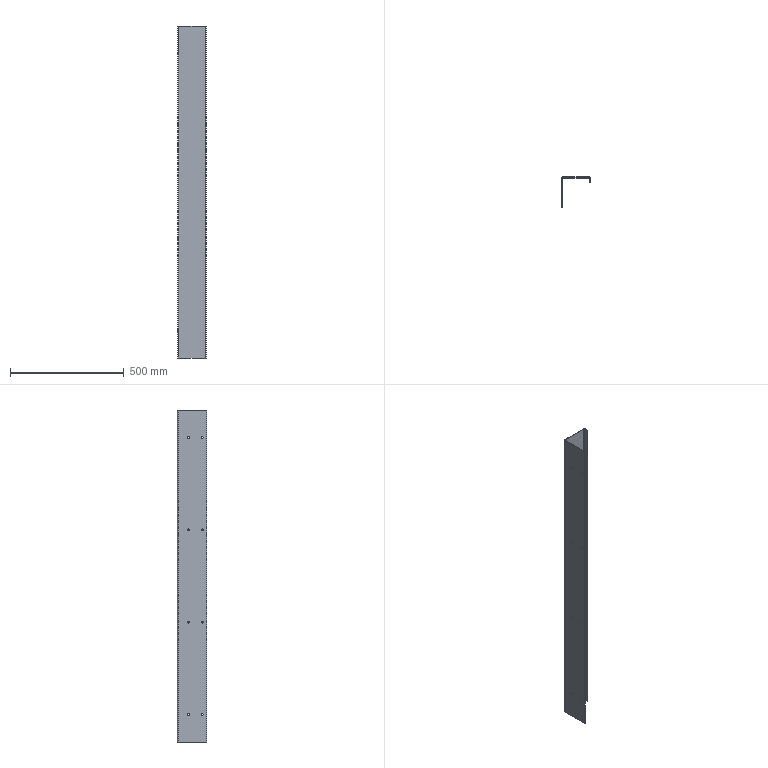Part | SolidWorks | features Extrusion 1, ICE 1 | 1 solid | 30 faces | box 126 x 130 x 1460 mm | volume 1168234 mm3 | cylinder 20 | plane 10 | commonest cylinder face diameters 8 x16 4 x2 10 x2
STEP:
#1=CARTESIAN_POINT('',(3.,80.,1335.));
#2=VERTEX_POINT('',#1);
#3=CARTESIAN_POINT('',(3.,80.,1343.));
#4=VERTEX_POINT('',#3);
#5=CARTESIAN_POINT('',(3.,80.,1339.));
#6=DIRECTION('',(-1.,0.,0.));
#7=DIRECTION('',(0.,0.,1.));
#8=AXIS2_PLACEMENT_3D('',#5,#6,#7);
#9=CIRCLE('',#8,4.);
#10=EDGE_CURVE('',#2,#4,#9,.T.);
#11=ORIENTED_EDGE('',*,*,#10,.F.);
#12=CARTESIAN_POINT('',(0.,80.,1335.));
#13=VERTEX_POINT('',#12);
#14=CARTESIAN_POINT('',(1460.,80.,1335.));
#15=DIRECTION('',(-1.,0.,0.));
#16=VECTOR('',#15,1000.);
#17=LINE('',#14,#16);
#18=EDGE_CURVE('',#2,#13,#17,.T.);
#19=ORIENTED_EDGE('',*,*,#18,.T.);
#20=CARTESIAN_POINT('',(0.,80.,1343.));
#21=VERTEX_POINT('',#20);
#22=CARTESIAN_POINT('',(0.,80.,1339.));
#23=DIRECTION('',(-1.,0.,0.));
#24=DIRECTION('',(0.,0.,1.));
#25=AXIS2_PLACEMENT_3D('',#22,#23,#24);
#26=CIRCLE('',#25,4.);
#27=EDGE_CURVE('',#13,#21,#26,.T.);
#28=ORIENTED_EDGE('',*,*,#27,.T.);
#29=CARTESIAN_POINT('',(1460.,80.,1343.));
#30=DIRECTION('',(-1.,0.,0.));
#31=VECTOR('',#30,1000.);
#32=LINE('',#29,#31);
#33=EDGE_CURVE('',#4,#21,#32,.T.);
#34=ORIENTED_EDGE('',*,*,#33,.F.);
#35=EDGE_LOOP('',(#11,#19,#28,#34));
#36=FACE_OUTER_BOUND('',#35,.T.);
#37=CARTESIAN_POINT('',(1460.,80.,1339.));
#38=DIRECTION('',(-1.,0.,0.));
#39=DIRECTION('',(0.,0.,1.));
#40=AXIS2_PLACEMENT_3D('',#37,#38,#39);
#41=CYLINDRICAL_SURFACE('',#40,4.);
#42=ADVANCED_FACE('',(#36),#41,.F.);
#43=CARTESIAN_POINT('',(3.,80.,929.));
#44=VERTEX_POINT('',#43);
#45=CARTESIAN_POINT('',(3.,80.,937.));
#46=VERTEX_POINT('',#45);
#47=CARTESIAN_POINT('',(3.,80.,933.));
#48=DIRECTION('',(-1.,0.,0.));
#49=DIRECTION('',(0.,0.,1.));
#50=AXIS2_PLACEMENT_3D('',#47,#48,#49);
#51=CIRCLE('',#50,4.);
#52=EDGE_CURVE('',#44,#46,#51,.T.);
#53=ORIENTED_EDGE('',*,*,#52,.F.);
#54=CARTESIAN_POINT('',(0.,80.,929.));
#55=VERTEX_POINT('',#54);
#56=CARTESIAN_POINT('',(1460.,80.,929.));
#57=DIRECTION('',(-1.,0.,0.));
#58=VECTOR('',#57,1000.);
#59=LINE('',#56,#58);
#60=EDGE_CURVE('',#44,#55,#59,.T.);
#61=ORIENTED_EDGE('',*,*,#60,.T.);
#62=CARTESIAN_POINT('',(0.,80.,937.));
#63=VERTEX_POINT('',#62);
#64=CARTESIAN_POINT('',(0.,80.,933.));
#65=DIRECTION('',(-1.,0.,0.));
#66=DIRECTION('',(0.,0.,1.));
#67=AXIS2_PLACEMENT_3D('',#64,#65,#66);
#68=CIRCLE('',#67,4.);
#69=EDGE_CURVE('',#55,#63,#68,.T.);
#70=ORIENTED_EDGE('',*,*,#69,.T.);
#71=CARTESIAN_POINT('',(1460.,80.,937.));
#72=DIRECTION('',(-1.,0.,0.));
#73=VECTOR('',#72,1000.);
#74=LINE('',#71,#73);
#75=EDGE_CURVE('',#46,#63,#74,.T.);
#76=ORIENTED_EDGE('',*,*,#75,.F.);
#77=EDGE_LOOP('',(#53,#61,#70,#76));
#78=FACE_OUTER_BOUND('',#77,.T.);
#79=CARTESIAN_POINT('',(1460.,80.,933.));
#80=DIRECTION('',(-1.,0.,0.));
#81=DIRECTION('',(0.,0.,1.));
#82=AXIS2_PLACEMENT_3D('',#79,#80,#81);
#83=CYLINDRICAL_SURFACE('',#82,4.);
#84=ADVANCED_FACE('',(#78),#83,.F.);
#85=CARTESIAN_POINT('',(3.,80.,523.));
#86=VERTEX_POINT('',#85);
#87=CARTESIAN_POINT('',(3.,80.,531.));
#88=VERTEX_POINT('',#87);
#89=CARTESIAN_POINT('',(3.,80.,527.));
#90=DIRECTION('',(-1.,0.,0.));
#91=DIRECTION('',(0.,0.,1.));
#92=AXIS2_PLACEMENT_3D('',#89,#90,#91);
#93=CIRCLE('',#92,4.);
#94=EDGE_CURVE('',#86,#88,#93,.T.);
#95=ORIENTED_EDGE('',*,*,#94,.F.);
#96=CARTESIAN_POINT('',(0.,80.,523.));
#97=VERTEX_POINT('',#96);
#98=CARTESIAN_POINT('',(1460.,80.,523.));
#99=DIRECTION('',(-1.,0.,0.));
#100=VECTOR('',#99,1000.);
#101=LINE('',#98,#100);
#102=EDGE_CURVE('',#86,#97,#101,.T.);
#103=ORIENTED_EDGE('',*,*,#102,.T.);
#104=CARTESIAN_POINT('',(0.,80.,531.));
#105=VERTEX_POINT('',#104);
#106=CARTESIAN_POINT('',(0.,80.,527.));
#107=DIRECTION('',(-1.,0.,0.));
#108=DIRECTION('',(0.,0.,1.));
#109=AXIS2_PLACEMENT_3D('',#106,#107,#108);
#110=CIRCLE('',#109,4.);
#111=EDGE_CURVE('',#97,#105,#110,.T.);
#112=ORIENTED_EDGE('',*,*,#111,.T.);
#113=CARTESIAN_POINT('',(1460.,80.,531.));
#114=DIRECTION('',(-1.,0.,0.));
#115=VECTOR('',#114,1000.);
#116=LINE('',#113,#115);
#117=EDGE_CURVE('',#88,#105,#116,.T.);
#118=ORIENTED_EDGE('',*,*,#117,.F.);
#119=EDGE_LOOP('',(#95,#103,#112,#118));
#120=FACE_OUTER_BOUND('',#119,.T.);
#121=CARTESIAN_POINT('',(1460.,80.,527.));
#122=DIRECTION('',(-1.,0.,0.));
#123=DIRECTION('',(0.,0.,1.));
#124=AXIS2_PLACEMENT_3D('',#121,#122,#123);
#125=CYLINDRICAL_SURFACE('',#124,4.);
#126=ADVANCED_FACE('',(#120),#125,.F.);
#127=CARTESIAN_POINT('',(3.,20.,117.));
#128=VERTEX_POINT('',#127);
#129=CARTESIAN_POINT('',(3.,20.,125.));
#130=VERTEX_POINT('',#129);
#131=CARTESIAN_POINT('',(3.,20.,121.));
#132=DIRECTION('',(-1.,0.,0.));
#133=DIRECTION('',(0.,0.,1.));
#134=AXIS2_PLACEMENT_3D('',#131,#132,#133);
#135=CIRCLE('',#134,4.);
#136=EDGE_CURVE('',#128,#130,#135,.T.);
#137=ORIENTED_EDGE('',*,*,#136,.F.);
#138=CARTESIAN_POINT('',(0.,20.,117.));
#139=VERTEX_POINT('',#138);
#140=CARTESIAN_POINT('',(1460.,20.,117.));
#141=DIRECTION('',(-1.,0.,0.));
#142=VECTOR('',#141,1000.);
#143=LINE('',#140,#142);
#144=EDGE_CURVE('',#128,#139,#143,.T.);
#145=ORIENTED_EDGE('',*,*,#144,.T.);
#146=CARTESIAN_POINT('',(0.,20.,125.));
#147=VERTEX_POINT('',#146);
#148=CARTESIAN_POINT('',(0.,20.,121.));
#149=DIRECTION('',(-1.,0.,0.));
#150=DIRECTION('',(0.,0.,1.));
#151=AXIS2_PLACEMENT_3D('',#148,#149,#150);
#152=CIRCLE('',#151,4.);
#153=EDGE_CURVE('',#139,#147,#152,.T.);
#154=ORIENTED_EDGE('',*,*,#153,.T.);
#155=CARTESIAN_POINT('',(1460.,20.,125.));
#156=DIRECTION('',(-1.,0.,0.));
#157=VECTOR('',#156,1000.);
#158=LINE('',#155,#157);
#159=EDGE_CURVE('',#130,#147,#158,.T.);
#160=ORIENTED_EDGE('',*,*,#159,.F.);
#161=EDGE_LOOP('',(#137,#145,#154,#160));
#162=FACE_OUTER_BOUND('',#161,.T.);
#163=CARTESIAN_POINT('',(1460.,20.,121.));
#164=DIRECTION('',(-1.,0.,0.));
#165=DIRECTION('',(0.,0.,1.));
#166=AXIS2_PLACEMENT_3D('',#163,#164,#165);
#167=CYLINDRICAL_SURFACE('',#166,4.);
#168=ADVANCED_FACE('',(#162),#167,.F.);
#169=CARTESIAN_POINT('',(3.,20.,1335.));
#170=VERTEX_POINT('',#169);
#171=CARTESIAN_POINT('',(3.,20.,1343.));
#172=VERTEX_POINT('',#171);
#173=CARTESIAN_POINT('',(3.,20.,1339.));
#174=DIRECTION('',(-1.,0.,0.));
#175=DIRECTION('',(0.,0.,1.));
#176=AXIS2_PLACEMENT_3D('',#173,#174,#175);
#177=CIRCLE('',#176,4.);
#178=EDGE_CURVE('',#170,#172,#177,.T.);
#179=ORIENTED_EDGE('',*,*,#178,.F.);
#180=CARTESIAN_POINT('',(0.,20.,1335.));
#181=VERTEX_POINT('',#180);
#182=CARTESIAN_POINT('',(1460.,20.,1335.));
#183=DIRECTION('',(-1.,0.,0.));
#184=VECTOR('',#183,1000.);
#185=LINE('',#182,#184);
#186=EDGE_CURVE('',#170,#181,#185,.T.);
#187=ORIENTED_EDGE('',*,*,#186,.T.);
#188=CARTESIAN_POINT('',(0.,20.,1343.));
#189=VERTEX_POINT('',#188);
#190=CARTESIAN_POINT('',(0.,20.,1339.));
#191=DIRECTION('',(-1.,0.,0.));
#192=DIRECTION('',(0.,0.,1.));
#193=AXIS2_PLACEMENT_3D('',#190,#191,#192);
#194=CIRCLE('',#193,4.);
#195=EDGE_CURVE('',#181,#189,#194,.T.);
#196=ORIENTED_EDGE('',*,*,#195,.T.);
#197=CARTESIAN_POINT('',(1460.,20.,1343.));
#198=DIRECTION('',(-1.,0.,0.));
#199=VECTOR('',#198,1000.);
#200=LINE('',#197,#199);
#201=EDGE_CURVE('',#172,#189,#200,.T.);
#202=ORIENTED_EDGE('',*,*,#201,.F.);
#203=EDGE_LOOP('',(#179,#187,#196,#202));
#204=FACE_OUTER_BOUND('',#203,.T.);
#205=CARTESIAN_POINT('',(1460.,20.,1339.));
#206=DIRECTION('',(-1.,0.,0.));
#207=DIRECTION('',(0.,0.,1.));
#208=AXIS2_PLACEMENT_3D('',#205,#206,#207);
#209=CYLINDRICAL_SURFACE('',#208,4.);
#210=ADVANCED_FACE('',(#204),#209,.F.);
#211=CARTESIAN_POINT('',(3.,20.,929.));
#212=VERTEX_POINT('',#211);
#213=CARTESIAN_POINT('',(3.,20.,937.));
#214=VERTEX_POINT('',#213);
#215=CARTESIAN_POINT('',(3.,20.,933.));
#216=DIRECTION('',(-1.,0.,0.));
#217=DIRECTION('',(0.,0.,1.));
#218=AXIS2_PLACEMENT_3D('',#215,#216,#217);
#219=CIRCLE('',#218,4.);
#220=EDGE_CURVE('',#212,#214,#219,.T.);
#221=ORIENTED_EDGE('',*,*,#220,.F.);
#222=CARTESIAN_POINT('',(0.,20.,929.));
#223=VERTEX_POINT('',#222);
#224=CARTESIAN_POINT('',(1460.,20.,929.));
#225=DIRECTION('',(-1.,0.,0.));
#226=VECTOR('',#225,1000.);
#227=LINE('',#224,#226);
#228=EDGE_CURVE('',#212,#223,#227,.T.);
#229=ORIENTED_EDGE('',*,*,#228,.T.);
#230=CARTESIAN_POINT('',(0.,20.,937.));
#231=VERTEX_POINT('',#230);
#232=CARTESIAN_POINT('',(0.,20.,933.));
#233=DIRECTION('',(-1.,0.,0.));
#234=DIRECTION('',(0.,0.,1.));
#235=AXIS2_PLACEMENT_3D('',#232,#233,#234);
#236=CIRCLE('',#235,4.);
#237=EDGE_CURVE('',#223,#231,#236,.T.);
#238=ORIENTED_EDGE('',*,*,#237,.T.);
#239=CARTESIAN_POINT('',(1460.,20.,937.));
#240=DIRECTION('',(-1.,0.,0.));
#241=VECTOR('',#240,1000.);
#242=LINE('',#239,#241);
#243=EDGE_CURVE('',#214,#231,#242,.T.);
#244=ORIENTED_EDGE('',*,*,#243,.F.);
#245=EDGE_LOOP('',(#221,#229,#238,#244));
#246=FACE_OUTER_BOUND('',#245,.T.);
#247=CARTESIAN_POINT('',(1460.,20.,933.));
#248=DIRECTION('',(-1.,0.,0.));
#249=DIRECTION('',(0.,0.,1.));
#250=AXIS2_PLACEMENT_3D('',#247,#248,#249);
#251=CYLINDRICAL_SURFACE('',#250,4.);
#252=ADVANCED_FACE('',(#246),#251,.F.);
#253=CARTESIAN_POINT('',(3.,20.,523.));
#254=VERTEX_POINT('',#253);
#255=CARTESIAN_POINT('',(3.,20.,531.));
#256=VERTEX_POINT('',#255);
#257=CARTESIAN_POINT('',(3.,20.,527.));
#258=DIRECTION('',(-1.,0.,0.));
#259=DIRECTION('',(0.,0.,1.));
#260=AXIS2_PLACEMENT_3D('',#257,#258,#259);
#261=CIRCLE('',#260,4.);
#262=EDGE_CURVE('',#254,#256,#261,.T.);
#263=ORIENTED_EDGE('',*,*,#262,.F.);
#264=CARTESIAN_POINT('',(0.,20.,523.));
#265=VERTEX_POINT('',#264);
#266=CARTESIAN_POINT('',(1460.,20.,523.));
#267=DIRECTION('',(-1.,0.,0.));
#268=VECTOR('',#267,1000.);
#269=LINE('',#266,#268);
#270=EDGE_CURVE('',#254,#265,#269,.T.);
#271=ORIENTED_EDGE('',*,*,#270,.T.);
#272=CARTESIAN_POINT('',(0.,20.,531.));
#273=VERTEX_POINT('',#272);
#274=CARTESIAN_POINT('',(0.,20.,527.));
#275=DIRECTION('',(-1.,0.,0.));
#276=DIRECTION('',(0.,0.,1.));
#277=AXIS2_PLACEMENT_3D('',#274,#275,#276);
#278=CIRCLE('',#277,4.);
#279=EDGE_CURVE('',#265,#273,#278,.T.);
#280=ORIENTED_EDGE('',*,*,#279,.T.);
#281=CARTESIAN_POINT('',(1460.,20.,531.));
#282=DIRECTION('',(-1.,0.,0.));
#283=VECTOR('',#282,1000.);
#284=LINE('',#281,#283);
#285=EDGE_CURVE('',#256,#273,#284,.T.);
#286=ORIENTED_EDGE('',*,*,#285,.F.);
#287=EDGE_LOOP('',(#263,#271,#280,#286));
#288=FACE_OUTER_BOUND('',#287,.T.);
#289=CARTESIAN_POINT('',(1460.,20.,527.));
#290=DIRECTION('',(-1.,0.,0.));
#291=DIRECTION('',(0.,0.,1.));
#292=AXIS2_PLACEMENT_3D('',#289,#290,#291);
#293=CYLINDRICAL_SURFACE('',#292,4.);
#294=ADVANCED_FACE('',(#288),#293,.F.);
#295=CARTESIAN_POINT('',(3.,80.,117.));
#296=VERTEX_POINT('',#295);
#297=CARTESIAN_POINT('',(3.,80.,125.));
#298=VERTEX_POINT('',#297);
#299=CARTESIAN_POINT('',(3.,80.,121.));
#300=DIRECTION('',(-1.,0.,0.));
#301=DIRECTION('',(0.,0.,1.));
#302=AXIS2_PLACEMENT_3D('',#299,#300,#301);
#303=CIRCLE('',#302,4.);
#304=EDGE_CURVE('',#296,#298,#303,.T.);
#305=ORIENTED_EDGE('',*,*,#304,.F.);
#306=CARTESIAN_POINT('',(0.,80.,117.));
#307=VERTEX_POINT('',#306);
#308=CARTESIAN_POINT('',(1460.,80.,117.));
#309=DIRECTION('',(-1.,0.,0.));
#310=VECTOR('',#309,1000.);
#311=LINE('',#308,#310);
#312=EDGE_CURVE('',#296,#307,#311,.T.);
#313=ORIENTED_EDGE('',*,*,#312,.T.);
#314=CARTESIAN_POINT('',(0.,80.,125.));
#315=VERTEX_POINT('',#314);
#316=CARTESIAN_POINT('',(0.,80.,121.));
#317=DIRECTION('',(-1.,0.,0.));
#318=DIRECTION('',(0.,0.,1.));
#319=AXIS2_PLACEMENT_3D('',#316,#317,#318);
#320=CIRCLE('',#319,4.);
#321=EDGE_CURVE('',#307,#315,#320,.T.);
#322=ORIENTED_EDGE('',*,*,#321,.T.);
#323=CARTESIAN_POINT('',(1460.,80.,125.));
#324=DIRECTION('',(-1.,0.,0.));
#325=VECTOR('',#324,1000.);
#326=LINE('',#323,#325);
#327=EDGE_CURVE('',#298,#315,#326,.T.);
#328=ORIENTED_EDGE('',*,*,#327,.F.);
#329=EDGE_LOOP('',(#305,#313,#322,#328));
#330=FACE_OUTER_BOUND('',#329,.T.);
#331=CARTESIAN_POINT('',(1460.,80.,121.));
#332=DIRECTION('',(-1.,0.,0.));
#333=DIRECTION('',(0.,0.,1.));
#334=AXIS2_PLACEMENT_3D('',#331,#332,#333);
#335=CYLINDRICAL_SURFACE('',#334,4.);
#336=ADVANCED_FACE('',(#330),#335,.F.);
#337=CARTESIAN_POINT('',(0.,80.,1339.));
#338=DIRECTION('',(-1.,0.,0.));
#339=DIRECTION('',(0.,0.,1.));
#340=AXIS2_PLACEMENT_3D('',#337,#338,#339);
#341=CIRCLE('',#340,4.);
#342=EDGE_CURVE('',#21,#13,#341,.T.);
#343=ORIENTED_EDGE('',*,*,#342,.F.);
#344=ORIENTED_EDGE('',*,*,#27,.F.);
#345=EDGE_LOOP('',(#343,#344));
#346=FACE_BOUND('',#345,.T.);
#347=CARTESIAN_POINT('',(0.,80.,933.));
#348=DIRECTION('',(-1.,0.,0.));
#349=DIRECTION('',(0.,0.,1.));
#350=AXIS2_PLACEMENT_3D('',#347,#348,#349);
#351=CIRCLE('',#350,4.);
#352=EDGE_CURVE('',#63,#55,#351,.T.);
#353=ORIENTED_EDGE('',*,*,#352,.F.);
#354=ORIENTED_EDGE('',*,*,#69,.F.);
#355=EDGE_LOOP('',(#353,#354));
#356=FACE_BOUND('',#355,.T.);
#357=CARTESIAN_POINT('',(0.,80.,527.));
#358=DIRECTION('',(-1.,0.,0.));
#359=DIRECTION('',(0.,0.,1.));
#360=AXIS2_PLACEMENT_3D('',#357,#358,#359);
#361=CIRCLE('',#360,4.);
#362=EDGE_CURVE('',#105,#97,#361,.T.);
#363=ORIENTED_EDGE('',*,*,#362,.F.);
#364=ORIENTED_EDGE('',*,*,#111,.F.);
#365=EDGE_LOOP('',(#363,#364));
#366=FACE_BOUND('',#365,.T.);
#367=CARTESIAN_POINT('',(0.,20.,121.));
#368=DIRECTION('',(-1.,0.,0.));
#369=DIRECTION('',(0.,0.,1.));
#370=AXIS2_PLACEMENT_3D('',#367,#368,#369);
#371=CIRCLE('',#370,4.);
#372=EDGE_CURVE('',#147,#139,#371,.T.);
#373=ORIENTED_EDGE('',*,*,#372,.F.);
#374=ORIENTED_EDGE('',*,*,#153,.F.);
#375=EDGE_LOOP('',(#373,#374));
#376=FACE_BOUND('',#375,.T.);
#377=CARTESIAN_POINT('',(0.,20.,1339.));
#378=DIRECTION('',(-1.,0.,0.));
#379=DIRECTION('',(0.,0.,1.));
#380=AXIS2_PLACEMENT_3D('',#377,#378,#379);
#381=CIRCLE('',#380,4.);
#382=EDGE_CURVE('',#189,#181,#381,.T.);
#383=ORIENTED_EDGE('',*,*,#382,.F.);
#384=ORIENTED_EDGE('',*,*,#195,.F.);
#385=EDGE_LOOP('',(#383,#384));
#386=FACE_BOUND('',#385,.T.);
#387=CARTESIAN_POINT('',(0.,20.,933.));
#388=DIRECTION('',(-1.,0.,0.));
#389=DIRECTION('',(0.,0.,1.));
#390=AXIS2_PLACEMENT_3D('',#387,#388,#389);
#391=CIRCLE('',#390,4.);
#392=EDGE_CURVE('',#231,#223,#391,.T.);
#393=ORIENTED_EDGE('',*,*,#392,.F.);
#394=ORIENTED_EDGE('',*,*,#237,.F.);
#395=EDGE_LOOP('',(#393,#394));
#396=FACE_BOUND('',#395,.T.);
#397=CARTESIAN_POINT('',(0.,20.,527.));
#398=DIRECTION('',(-1.,0.,0.));
#399=DIRECTION('',(0.,0.,1.));
#400=AXIS2_PLACEMENT_3D('',#397,#398,#399);
#401=CIRCLE('',#400,4.);
#402=EDGE_CURVE('',#273,#265,#401,.T.);
#403=ORIENTED_EDGE('',*,*,#402,.F.);
#404=ORIENTED_EDGE('',*,*,#279,.F.);
#405=EDGE_LOOP('',(#403,#404));
#406=FACE_BOUND('',#405,.T.);
#407=CARTESIAN_POINT('',(0.,80.,121.));
#408=DIRECTION('',(-1.,0.,0.));
#409=DIRECTION('',(0.,0.,1.));
#410=AXIS2_PLACEMENT_3D('',#407,#408,#409);
#411=CIRCLE('',#410,4.);
#412=EDGE_CURVE('',#315,#307,#411,.T.);
#413=ORIENTED_EDGE('',*,*,#412,.F.);
#414=ORIENTED_EDGE('',*,*,#321,.F.);
#415=EDGE_LOOP('',(#413,#414));
#416=FACE_BOUND('',#415,.T.);
#417=CARTESIAN_POINT('',(0.,0.,0.));
#418=VERTEX_POINT('',#417);
#419=CARTESIAN_POINT('',(0.,125.,0.));
#420=VERTEX_POINT('',#419);
#421=CARTESIAN_POINT('',(0.,0.,0.));
#422=DIRECTION('',(0.,1.,0.));
#423=VECTOR('',#422,1000.);
#424=LINE('',#421,#423);
#425=EDGE_CURVE('',#418,#420,#424,.T.);
#426=ORIENTED_EDGE('',*,*,#425,.F.);
#427=CARTESIAN_POINT('',(0.,0.,1460.));
#428=VERTEX_POINT('',#427);
#429=CARTESIAN_POINT('',(0.,0.,1460.));
#430=DIRECTION('',(0.,0.,-1.));
#431=VECTOR('',#430,1000.);
#432=LINE('',#429,#431);
#433=EDGE_CURVE('',#428,#418,#432,.T.);
#434=ORIENTED_EDGE('',*,*,#433,.F.);
#435=CARTESIAN_POINT('',(0.,125.,1460.));
#436=VERTEX_POINT('',#435);
#437=CARTESIAN_POINT('',(0.,0.,1460.));
#438=DIRECTION('',(0.,1.,0.));
#439=VECTOR('',#438,1000.);
#440=LINE('',#437,#439);
#441=EDGE_CURVE('',#428,#436,#440,.T.);
#442=ORIENTED_EDGE('',*,*,#441,.T.);
#443=CARTESIAN_POINT('',(0.,125.,1460.));
#444=DIRECTION('',(0.,0.,-1.));
#445=VECTOR('',#444,1000.);
#446=LINE('',#443,#445);
#447=EDGE_CURVE('',#436,#420,#446,.T.);
#448=ORIENTED_EDGE('',*,*,#447,.T.);
#449=EDGE_LOOP('',(#426,#434,#442,#448));
#450=FACE_OUTER_BOUND('',#449,.T.);
#451=CARTESIAN_POINT('',(0.,0.,1460.));
#452=DIRECTION('',(-1.,0.,0.));
#453=DIRECTION('',(0.,0.,1.));
#454=AXIS2_PLACEMENT_3D('',#451,#452,#453);
#455=PLANE('',#454);
#456=ADVANCED_FACE('',(#346,#356,#366,#376,#386,#396,#406,#416,#450),#455,.T.);
#457=CARTESIAN_POINT('',(3.,0.,0.));
#458=VERTEX_POINT('',#457);
#459=CARTESIAN_POINT('',(0.,0.,0.));
#460=DIRECTION('',(1.,0.,0.));
#461=VECTOR('',#460,1000.);
#462=LINE('',#459,#461);
#463=EDGE_CURVE('',#418,#458,#462,.T.);
#464=ORIENTED_EDGE('',*,*,#463,.T.);
#465=CARTESIAN_POINT('',(3.,0.,1460.));
#466=VERTEX_POINT('',#465);
#467=CARTESIAN_POINT('',(3.,0.,1460.));
#468=DIRECTION('',(0.,0.,-1.));
#469=VECTOR('',#468,1000.);
#470=LINE('',#467,#469);
#471=EDGE_CURVE('',#466,#458,#470,.T.);
#472=ORIENTED_EDGE('',*,*,#471,.F.);
#473=CARTESIAN_POINT('',(0.,0.,1460.));
#474=DIRECTION('',(1.,0.,0.));
#475=VECTOR('',#474,1000.);
#476=LINE('',#473,#475);
#477=EDGE_CURVE('',#428,#466,#476,.T.);
#478=ORIENTED_EDGE('',*,*,#477,.F.);
#479=ORIENTED_EDGE('',*,*,#433,.T.);
#480=EDGE_LOOP('',(#464,#472,#478,#479));
#481=FACE_OUTER_BOUND('',#480,.T.);
#482=CARTESIAN_POINT('',(0.,0.,1460.));
#483=DIRECTION('',(0.,1.,0.));
#484=DIRECTION('',(0.,0.,1.));
#485=AXIS2_PLACEMENT_3D('',#482,#483,#484);
#486=PLANE('',#485);
#487=ADVANCED_FACE('',(#481),#486,.F.);
#488=CARTESIAN_POINT('',(3.,80.,1339.));
#489=DIRECTION('',(-1.,0.,0.));
#490=DIRECTION('',(0.,0.,1.));
#491=AXIS2_PLACEMENT_3D('',#488,#489,#490);
#492=CIRCLE('',#491,4.);
#493=EDGE_CURVE('',#4,#2,#492,.T.);
#494=ORIENTED_EDGE('',*,*,#493,.T.);
#495=ORIENTED_EDGE('',*,*,#10,.T.);
#496=EDGE_LOOP('',(#494,#495));
#497=FACE_BOUND('',#496,.T.);
#498=CARTESIAN_POINT('',(3.,80.,933.));
#499=DIRECTION('',(-1.,0.,0.));
#500=DIRECTION('',(0.,0.,1.));
#501=AXIS2_PLACEMENT_3D('',#498,#499,#500);
#502=CIRCLE('',#501,4.);
#503=EDGE_CURVE('',#46,#44,#502,.T.);
#504=ORIENTED_EDGE('',*,*,#503,.T.);
#505=ORIENTED_EDGE('',*,*,#52,.T.);
#506=EDGE_LOOP('',(#504,#505));
#507=FACE_BOUND('',#506,.T.);
#508=CARTESIAN_POINT('',(3.,80.,527.));
#509=DIRECTION('',(-1.,0.,0.));
#510=DIRECTION('',(0.,0.,1.));
#511=AXIS2_PLACEMENT_3D('',#508,#509,#510);
#512=CIRCLE('',#511,4.);
#513=EDGE_CURVE('',#88,#86,#512,.T.);
#514=ORIENTED_EDGE('',*,*,#513,.T.);
#515=ORIENTED_EDGE('',*,*,#94,.T.);
#516=EDGE_LOOP('',(#514,#515));
#517=FACE_BOUND('',#516,.T.);
#518=CARTESIAN_POINT('',(3.,20.,121.));
#519=DIRECTION('',(-1.,0.,0.));
#520=DIRECTION('',(0.,0.,1.));
#521=AXIS2_PLACEMENT_3D('',#518,#519,#520);
#522=CIRCLE('',#521,4.);
#523=EDGE_CURVE('',#130,#128,#522,.T.);
#524=ORIENTED_EDGE('',*,*,#523,.T.);
#525=ORIENTED_EDGE('',*,*,#136,.T.);
#526=EDGE_LOOP('',(#524,#525));
#527=FACE_BOUND('',#526,.T.);
#528=CARTESIAN_POINT('',(3.,20.,1339.));
#529=DIRECTION('',(-1.,0.,0.));
#530=DIRECTION('',(0.,0.,1.));
#531=AXIS2_PLACEMENT_3D('',#528,#529,#530);
#532=CIRCLE('',#531,4.);
#533=EDGE_CURVE('',#172,#170,#532,.T.);
#534=ORIENTED_EDGE('',*,*,#533,.T.);
#535=ORIENTED_EDGE('',*,*,#178,.T.);
#536=EDGE_LOOP('',(#534,#535));
#537=FACE_BOUND('',#536,.T.);
#538=CARTESIAN_POINT('',(3.,20.,933.));
#539=DIRECTION('',(-1.,0.,0.));
#540=DIRECTION('',(0.,0.,1.));
#541=AXIS2_PLACEMENT_3D('',#538,#539,#540);
#542=CIRCLE('',#541,4.);
#543=EDGE_CURVE('',#214,#212,#542,.T.);
#544=ORIENTED_EDGE('',*,*,#543,.T.);
#545=ORIENTED_EDGE('',*,*,#220,.T.);
#546=EDGE_LOOP('',(#544,#545));
#547=FACE_BOUND('',#546,.T.);
#548=CARTESIAN_POINT('',(3.,20.,527.));
#549=DIRECTION('',(-1.,0.,0.));
#550=DIRECTION('',(0.,0.,1.));
#551=AXIS2_PLACEMENT_3D('',#548,#549,#550);
#552=CIRCLE('',#551,4.);
#553=EDGE_CURVE('',#256,#254,#552,.T.);
#554=ORIENTED_EDGE('',*,*,#553,.T.);
#555=ORIENTED_EDGE('',*,*,#262,.T.);
#556=EDGE_LOOP('',(#554,#555));
#557=FACE_BOUND('',#556,.T.);
#558=CARTESIAN_POINT('',(3.,80.,121.));
#559=DIRECTION('',(-1.,0.,0.));
#560=DIRECTION('',(0.,0.,1.));
#561=AXIS2_PLACEMENT_3D('',#558,#559,#560);
#562=CIRCLE('',#561,4.);
#563=EDGE_CURVE('',#298,#296,#562,.T.);
#564=ORIENTED_EDGE('',*,*,#563,.T.);
#565=ORIENTED_EDGE('',*,*,#304,.T.);
#566=EDGE_LOOP('',(#564,#565));
#567=FACE_BOUND('',#566,.T.);
#568=CARTESIAN_POINT('',(3.,125.,0.));
#569=VERTEX_POINT('',#568);
#570=CARTESIAN_POINT('',(3.,0.,0.));
#571=DIRECTION('',(0.,1.,0.));
#572=VECTOR('',#571,1000.);
#573=LINE('',#570,#572);
#574=EDGE_CURVE('',#458,#569,#573,.T.);
#575=ORIENTED_EDGE('',*,*,#574,.T.);
#576=CARTESIAN_POINT('',(3.,125.,1460.));
#577=VERTEX_POINT('',#576);
#578=CARTESIAN_POINT('',(3.,125.,1460.));
#579=DIRECTION('',(0.,0.,-1.));
#580=VECTOR('',#579,1000.);
#581=LINE('',#578,#580);
#582=EDGE_CURVE('',#577,#569,#581,.T.);
#583=ORIENTED_EDGE('',*,*,#582,.F.);
#584=CARTESIAN_POINT('',(3.,0.,1460.));
#585=DIRECTION('',(0.,1.,0.));
#586=VECTOR('',#585,1000.);
#587=LINE('',#584,#586);
#588=EDGE_CURVE('',#466,#577,#587,.T.);
#589=ORIENTED_EDGE('',*,*,#588,.F.);
#590=ORIENTED_EDGE('',*,*,#471,.T.);
#591=EDGE_LOOP('',(#575,#583,#589,#590));
#592=FACE_OUTER_BOUND('',#591,.T.);
#593=CARTESIAN_POINT('',(3.,0.,1460.));
#594=DIRECTION('',(-1.,0.,0.));
#595=DIRECTION('',(0.,0.,1.));
#596=AXIS2_PLACEMENT_3D('',#593,#594,#595);
#597=PLANE('',#596);
#598=ADVANCED_FACE('',(#497,#507,#517,#527,#537,#547,#557,#567,#592),#597,.F.);
#599=CARTESIAN_POINT('',(5.,127.,0.));
#600=VERTEX_POINT('',#599);
#601=CARTESIAN_POINT('',(5.,125.,0.));
#602=DIRECTION('',(0.,0.,-1.));
#603=DIRECTION('',(-1.,0.,0.));
#604=AXIS2_PLACEMENT_3D('',#601,#602,#603);
#605=CIRCLE('',#604,2.);
#606=EDGE_CURVE('',#569,#600,#605,.T.);
#607=ORIENTED_EDGE('',*,*,#606,.T.);
#608=CARTESIAN_POINT('',(5.,127.,1460.));
#609=VERTEX_POINT('',#608);
#610=CARTESIAN_POINT('',(5.,127.,1460.));
#611=DIRECTION('',(0.,0.,-1.));
#612=VECTOR('',#611,1000.);
#613=LINE('',#610,#612);
#614=EDGE_CURVE('',#609,#600,#613,.T.);
#615=ORIENTED_EDGE('',*,*,#614,.F.);
#616=CARTESIAN_POINT('',(5.,125.,1460.));
#617=DIRECTION('',(0.,0.,-1.));
#618=DIRECTION('',(-1.,0.,0.));
#619=AXIS2_PLACEMENT_3D('',#616,#617,#618);
#620=CIRCLE('',#619,2.);
#621=EDGE_CURVE('',#577,#609,#620,.T.);
#622=ORIENTED_EDGE('',*,*,#621,.F.);
#623=ORIENTED_EDGE('',*,*,#582,.T.);
#624=EDGE_LOOP('',(#607,#615,#622,#623));
#625=FACE_OUTER_BOUND('',#624,.T.);
#626=CARTESIAN_POINT('',(5.,125.,1460.));
#627=DIRECTION('',(0.,0.,-1.));
#628=DIRECTION('',(-1.,0.,0.));
#629=AXIS2_PLACEMENT_3D('',#626,#627,#628);
#630=CYLINDRICAL_SURFACE('',#629,2.);
#631=ADVANCED_FACE('',(#625),#630,.F.);
#632=CARTESIAN_POINT('',(121.,127.,0.));
#633=VERTEX_POINT('',#632);
#634=CARTESIAN_POINT('',(5.,127.,0.));
#635=DIRECTION('',(1.,0.,0.));
#636=VECTOR('',#635,1000.);
#637=LINE('',#634,#636);
#638=EDGE_CURVE('',#600,#633,#637,.T.);
#639=ORIENTED_EDGE('',*,*,#638,.T.);
#640=CARTESIAN_POINT('',(121.,127.,1460.));
#641=VERTEX_POINT('',#640);
#642=CARTESIAN_POINT('',(121.,127.,1460.));
#643=DIRECTION('',(0.,0.,-1.));
#644=VECTOR('',#643,1000.);
#645=LINE('',#642,#644);
#646=EDGE_CURVE('',#641,#633,#645,.T.);
#647=ORIENTED_EDGE('',*,*,#646,.F.);
#648=CARTESIAN_POINT('',(5.,127.,1460.));
#649=DIRECTION('',(1.,0.,0.));
#650=VECTOR('',#649,1000.);
#651=LINE('',#648,#650);
#652=EDGE_CURVE('',#609,#641,#651,.T.);
#653=ORIENTED_EDGE('',*,*,#652,.F.);
#654=ORIENTED_EDGE('',*,*,#614,.T.);
#655=EDGE_LOOP('',(#639,#647,#653,#654));
#656=FACE_OUTER_BOUND('',#655,.T.);
#657=CARTESIAN_POINT('',(5.,127.,1460.));
#658=DIRECTION('',(0.,1.,0.));
#659=DIRECTION('',(0.,0.,1.));
#660=AXIS2_PLACEMENT_3D('',#657,#658,#659);
#661=PLANE('',#660);
#662=ADVANCED_FACE('',(#656),#661,.F.);
#663=CARTESIAN_POINT('',(123.,125.,0.));
#664=VERTEX_POINT('',#663);
#665=CARTESIAN_POINT('',(121.,125.,0.));
#666=DIRECTION('',(0.,0.,-1.));
#667=DIRECTION('',(-1.,0.,0.));
#668=AXIS2_PLACEMENT_3D('',#665,#666,#667);
#669=CIRCLE('',#668,2.);
#670=EDGE_CURVE('',#633,#664,#669,.T.);
#671=ORIENTED_EDGE('',*,*,#670,.T.);
#672=CARTESIAN_POINT('',(123.,125.,1460.));
#673=VERTEX_POINT('',#672);
#674=CARTESIAN_POINT('',(123.,125.,1460.));
#675=DIRECTION('',(0.,0.,-1.));
#676=VECTOR('',#675,1000.);
#677=LINE('',#674,#676);
#678=EDGE_CURVE('',#673,#664,#677,.T.);
#679=ORIENTED_EDGE('',*,*,#678,.F.);
#680=CARTESIAN_POINT('',(121.,125.,1460.));
#681=DIRECTION('',(0.,0.,-1.));
#682=DIRECTION('',(-1.,0.,0.));
#683=AXIS2_PLACEMENT_3D('',#680,#681,#682);
#684=CIRCLE('',#683,2.);
#685=EDGE_CURVE('',#641,#673,#684,.T.);
#686=ORIENTED_EDGE('',*,*,#685,.F.);
#687=ORIENTED_EDGE('',*,*,#646,.T.);
#688=EDGE_LOOP('',(#671,#679,#686,#687));
#689=FACE_OUTER_BOUND('',#688,.T.);
#690=CARTESIAN_POINT('',(121.,125.,1460.));
#691=DIRECTION('',(0.,0.,-1.));
#692=DIRECTION('',(-1.,0.,0.));
#693=AXIS2_PLACEMENT_3D('',#690,#691,#692);
#694=CYLINDRICAL_SURFACE('',#693,2.);
#695=ADVANCED_FACE('',(#689),#694,.F.);
#696=CARTESIAN_POINT('',(123.,110.,0.));
#697=VERTEX_POINT('',#696);
#698=CARTESIAN_POINT('',(123.,125.,0.));
#699=DIRECTION('',(0.,-1.,0.));
#700=VECTOR('',#699,1000.);
#701=LINE('',#698,#700);
#702=EDGE_CURVE('',#664,#697,#701,.T.);
#703=ORIENTED_EDGE('',*,*,#702,.T.);
#704=CARTESIAN_POINT('',(123.,110.,1460.));
#705=VERTEX_POINT('',#704);
#706=CARTESIAN_POINT('',(123.,110.,1460.));
#707=DIRECTION('',(0.,0.,-1.));
#708=VECTOR('',#707,1000.);
#709=LINE('',#706,#708);
#710=EDGE_CURVE('',#705,#697,#709,.T.);
#711=ORIENTED_EDGE('',*,*,#710,.F.);
#712=CARTESIAN_POINT('',(123.,125.,1460.));
#713=DIRECTION('',(0.,-1.,0.));
#714=VECTOR('',#713,1000.);
#715=LINE('',#712,#714);
#716=EDGE_CURVE('',#673,#705,#715,.T.);
#717=ORIENTED_EDGE('',*,*,#716,.F.);
#718=ORIENTED_EDGE('',*,*,#678,.T.);
#719=EDGE_LOOP('',(#703,#711,#717,#718));
#720=FACE_OUTER_BOUND('',#719,.T.);
#721=CARTESIAN_POINT('',(123.,125.,1460.));
#722=DIRECTION('',(1.,0.,0.));
#723=DIRECTION('',(0.,0.,-1.));
#724=AXIS2_PLACEMENT_3D('',#721,#722,#723);
#725=PLANE('',#724);
#726=ADVANCED_FACE('',(#720),#725,.F.);
#727=CARTESIAN_POINT('',(126.,110.,0.));
#728=VERTEX_POINT('',#727);
#729=CARTESIAN_POINT('',(126.,110.,0.));
#730=DIRECTION('',(-1.,0.,0.));
#731=VECTOR('',#730,1000.);
#732=LINE('',#729,#731);
#733=EDGE_CURVE('',#728,#697,#732,.T.);
#734=ORIENTED_EDGE('',*,*,#733,.F.);
#735=CARTESIAN_POINT('',(126.,110.,1460.));
#736=VERTEX_POINT('',#735);
#737=CARTESIAN_POINT('',(126.,110.,1460.));
#738=DIRECTION('',(0.,0.,-1.));
#739=VECTOR('',#738,1000.);
#740=LINE('',#737,#739);
#741=EDGE_CURVE('',#736,#728,#740,.T.);
#742=ORIENTED_EDGE('',*,*,#741,.F.);
#743=CARTESIAN_POINT('',(126.,110.,1460.));
#744=DIRECTION('',(-1.,0.,0.));
#745=VECTOR('',#744,1000.);
#746=LINE('',#743,#745);
#747=EDGE_CURVE('',#736,#705,#746,.T.);
#748=ORIENTED_EDGE('',*,*,#747,.T.);
#749=ORIENTED_EDGE('',*,*,#710,.T.);
#750=EDGE_LOOP('',(#734,#742,#748,#749));
#751=FACE_OUTER_BOUND('',#750,.T.);
#752=CARTESIAN_POINT('',(126.,110.,1460.));
#753=DIRECTION('',(0.,-1.,0.));
#754=DIRECTION('',(0.,0.,-1.));
#755=AXIS2_PLACEMENT_3D('',#752,#753,#754);
#756=PLANE('',#755);
#757=ADVANCED_FACE('',(#751),#756,.T.);
#758=CARTESIAN_POINT('',(126.,125.,0.));
#759=VERTEX_POINT('',#758);
#760=CARTESIAN_POINT('',(126.,125.,0.));
#761=DIRECTION('',(0.,-1.,0.));
#762=VECTOR('',#761,1000.);
#763=LINE('',#760,#762);
#764=EDGE_CURVE('',#759,#728,#763,.T.);
#765=ORIENTED_EDGE('',*,*,#764,.F.);
#766=CARTESIAN_POINT('',(126.,125.,1460.));
#767=VERTEX_POINT('',#766);
#768=CARTESIAN_POINT('',(126.,125.,1460.));
#769=DIRECTION('',(0.,0.,-1.));
#770=VECTOR('',#769,1000.);
#771=LINE('',#768,#770);
#772=EDGE_CURVE('',#767,#759,#771,.T.);
#773=ORIENTED_EDGE('',*,*,#772,.F.);
#774=CARTESIAN_POINT('',(126.,125.,1460.));
#775=DIRECTION('',(0.,-1.,0.));
#776=VECTOR('',#775,1000.);
#777=LINE('',#774,#776);
#778=EDGE_CURVE('',#767,#736,#777,.T.);
#779=ORIENTED_EDGE('',*,*,#778,.T.);
#780=ORIENTED_EDGE('',*,*,#741,.T.);
#781=EDGE_LOOP('',(#765,#773,#779,#780));
#782=FACE_OUTER_BOUND('',#781,.T.);
#783=CARTESIAN_POINT('',(126.,125.,1460.));
#784=DIRECTION('',(1.,0.,0.));
#785=DIRECTION('',(0.,0.,-1.));
#786=AXIS2_PLACEMENT_3D('',#783,#784,#785);
#787=PLANE('',#786);
#788=ADVANCED_FACE('',(#782),#787,.T.);
#789=CARTESIAN_POINT('',(121.,130.,0.));
#790=VERTEX_POINT('',#789);
#791=CARTESIAN_POINT('',(121.,125.,0.));
#792=DIRECTION('',(0.,0.,-1.));
#793=DIRECTION('',(-1.,0.,0.));
#794=AXIS2_PLACEMENT_3D('',#791,#792,#793);
#795=CIRCLE('',#794,5.);
#796=EDGE_CURVE('',#790,#759,#795,.T.);
#797=ORIENTED_EDGE('',*,*,#796,.F.);
#798=CARTESIAN_POINT('',(121.,130.,1460.));
#799=VERTEX_POINT('',#798);
#800=CARTESIAN_POINT('',(121.,130.,1460.));
#801=DIRECTION('',(0.,0.,-1.));
#802=VECTOR('',#801,1000.);
#803=LINE('',#800,#802);
#804=EDGE_CURVE('',#799,#790,#803,.T.);
#805=ORIENTED_EDGE('',*,*,#804,.F.);
#806=CARTESIAN_POINT('',(121.,125.,1460.));
#807=DIRECTION('',(0.,0.,-1.));
#808=DIRECTION('',(-1.,0.,0.));
#809=AXIS2_PLACEMENT_3D('',#806,#807,#808);
#810=CIRCLE('',#809,5.);
#811=EDGE_CURVE('',#799,#767,#810,.T.);
#812=ORIENTED_EDGE('',*,*,#811,.T.);
#813=ORIENTED_EDGE('',*,*,#772,.T.);
#814=EDGE_LOOP('',(#797,#805,#812,#813));
#815=FACE_OUTER_BOUND('',#814,.T.);
#816=CARTESIAN_POINT('',(121.,125.,1460.));
#817=DIRECTION('',(0.,0.,-1.));
#818=DIRECTION('',(-1.,0.,0.));
#819=AXIS2_PLACEMENT_3D('',#816,#817,#818);
#820=CYLINDRICAL_SURFACE('',#819,5.);
#821=ADVANCED_FACE('',(#815),#820,.T.);
#822=CARTESIAN_POINT('',(5.,130.,0.));
#823=VERTEX_POINT('',#822);
#824=CARTESIAN_POINT('',(5.,130.,0.));
#825=DIRECTION('',(1.,0.,0.));
#826=VECTOR('',#825,1000.);
#827=LINE('',#824,#826);
#828=EDGE_CURVE('',#823,#790,#827,.T.);
#829=ORIENTED_EDGE('',*,*,#828,.F.);
#830=CARTESIAN_POINT('',(5.,130.,1460.));
#831=VERTEX_POINT('',#830);
#832=CARTESIAN_POINT('',(5.,130.,1460.));
#833=DIRECTION('',(0.,0.,-1.));
#834=VECTOR('',#833,1000.);
#835=LINE('',#832,#834);
#836=EDGE_CURVE('',#831,#823,#835,.T.);
#837=ORIENTED_EDGE('',*,*,#836,.F.);
#838=CARTESIAN_POINT('',(5.,130.,1460.));
#839=DIRECTION('',(1.,0.,0.));
#840=VECTOR('',#839,1000.);
#841=LINE('',#838,#840);
#842=EDGE_CURVE('',#831,#799,#841,.T.);
#843=ORIENTED_EDGE('',*,*,#842,.T.);
#844=ORIENTED_EDGE('',*,*,#804,.T.);
#845=EDGE_LOOP('',(#829,#837,#843,#844));
#846=FACE_OUTER_BOUND('',#845,.T.);
#847=CARTESIAN_POINT('',(5.,130.,1460.));
#848=DIRECTION('',(0.,1.,0.));
#849=DIRECTION('',(0.,0.,1.));
#850=AXIS2_PLACEMENT_3D('',#847,#848,#849);
#851=PLANE('',#850);
#852=ADVANCED_FACE('',(#846),#851,.T.);
#853=CARTESIAN_POINT('',(5.,125.,0.));
#854=DIRECTION('',(0.,0.,-1.));
#855=DIRECTION('',(-1.,0.,0.));
#856=AXIS2_PLACEMENT_3D('',#853,#854,#855);
#857=CIRCLE('',#856,5.);
#858=EDGE_CURVE('',#420,#823,#857,.T.);
#859=ORIENTED_EDGE('',*,*,#858,.F.);
#860=ORIENTED_EDGE('',*,*,#447,.F.);
#861=CARTESIAN_POINT('',(5.,125.,1460.));
#862=DIRECTION('',(0.,0.,-1.));
#863=DIRECTION('',(-1.,0.,0.));
#864=AXIS2_PLACEMENT_3D('',#861,#862,#863);
#865=CIRCLE('',#864,5.);
#866=EDGE_CURVE('',#436,#831,#865,.T.);
#867=ORIENTED_EDGE('',*,*,#866,.T.);
#868=ORIENTED_EDGE('',*,*,#836,.T.);
#869=EDGE_LOOP('',(#859,#860,#867,#868));
#870=FACE_OUTER_BOUND('',#869,.T.);
#871=CARTESIAN_POINT('',(5.,125.,1460.));
#872=DIRECTION('',(0.,0.,-1.));
#873=DIRECTION('',(-1.,0.,0.));
#874=AXIS2_PLACEMENT_3D('',#871,#872,#873);
#875=CYLINDRICAL_SURFACE('',#874,5.);
#876=ADVANCED_FACE('',(#870),#875,.T.);
#877=ORIENTED_EDGE('',*,*,#441,.F.);
#878=ORIENTED_EDGE('',*,*,#477,.T.);
#879=ORIENTED_EDGE('',*,*,#588,.T.);
#880=ORIENTED_EDGE('',*,*,#621,.T.);
#881=ORIENTED_EDGE('',*,*,#652,.T.);
#882=ORIENTED_EDGE('',*,*,#685,.T.);
#883=ORIENTED_EDGE('',*,*,#716,.T.);
#884=ORIENTED_EDGE('',*,*,#747,.F.);
#885=ORIENTED_EDGE('',*,*,#778,.F.);
#886=ORIENTED_EDGE('',*,*,#811,.F.);
#887=ORIENTED_EDGE('',*,*,#842,.F.);
#888=ORIENTED_EDGE('',*,*,#866,.F.);
#889=EDGE_LOOP('',(#877,#878,#879,#880,#881,#882,#883,#884,#885,#886,#887,#888));
#890=FACE_OUTER_BOUND('',#889,.T.);
#891=CARTESIAN_POINT('',(5.,125.,1460.));
#892=DIRECTION('',(0.,0.,-1.));
#893=DIRECTION('',(-1.,0.,0.));
#894=AXIS2_PLACEMENT_3D('',#891,#892,#893);
#895=PLANE('',#894);
#896=ADVANCED_FACE('',(#890),#895,.F.);
#897=ORIENTED_EDGE('',*,*,#425,.T.);
#898=ORIENTED_EDGE('',*,*,#858,.T.);
#899=ORIENTED_EDGE('',*,*,#828,.T.);
#900=ORIENTED_EDGE('',*,*,#796,.T.);
#901=ORIENTED_EDGE('',*,*,#764,.T.);
#902=ORIENTED_EDGE('',*,*,#733,.T.);
#903=ORIENTED_EDGE('',*,*,#702,.F.);
#904=ORIENTED_EDGE('',*,*,#670,.F.);
#905=ORIENTED_EDGE('',*,*,#638,.F.);
#906=ORIENTED_EDGE('',*,*,#606,.F.);
#907=ORIENTED_EDGE('',*,*,#574,.F.);
#908=ORIENTED_EDGE('',*,*,#463,.F.);
#909=EDGE_LOOP('',(#897,#898,#899,#900,#901,#902,#903,#904,#905,#906,#907,#908));
#910=FACE_OUTER_BOUND('',#909,.T.);
#911=CARTESIAN_POINT('',(5.,125.,0.));
#912=DIRECTION('',(0.,0.,-1.));
#913=DIRECTION('',(-1.,0.,0.));
#914=AXIS2_PLACEMENT_3D('',#911,#912,#913);
#915=PLANE('',#914);
#916=ADVANCED_FACE('',(#910),#915,.T.);
#917=ORIENTED_EDGE('',*,*,#312,.F.);
#918=ORIENTED_EDGE('',*,*,#563,.F.);
#919=ORIENTED_EDGE('',*,*,#327,.T.);
#920=ORIENTED_EDGE('',*,*,#412,.T.);
#921=EDGE_LOOP('',(#917,#918,#919,#920));
#922=FACE_OUTER_BOUND('',#921,.T.);
#923=CARTESIAN_POINT('',(1460.,80.,121.));
#924=DIRECTION('',(-1.,0.,0.));
#925=DIRECTION('',(0.,0.,1.));
#926=AXIS2_PLACEMENT_3D('',#923,#924,#925);
#927=CYLINDRICAL_SURFACE('',#926,4.);
#928=ADVANCED_FACE('',(#922),#927,.F.);
#929=ORIENTED_EDGE('',*,*,#270,.F.);
#930=ORIENTED_EDGE('',*,*,#553,.F.);
#931=ORIENTED_EDGE('',*,*,#285,.T.);
#932=ORIENTED_EDGE('',*,*,#402,.T.);
#933=EDGE_LOOP('',(#929,#930,#931,#932));
#934=FACE_OUTER_BOUND('',#933,.T.);
#935=CARTESIAN_POINT('',(1460.,20.,527.));
#936=DIRECTION('',(-1.,0.,0.));
#937=DIRECTION('',(0.,0.,1.));
#938=AXIS2_PLACEMENT_3D('',#935,#936,#937);
#939=CYLINDRICAL_SURFACE('',#938,4.);
#940=ADVANCED_FACE('',(#934),#939,.F.);
#941=ORIENTED_EDGE('',*,*,#228,.F.);
#942=ORIENTED_EDGE('',*,*,#543,.F.);
#943=ORIENTED_EDGE('',*,*,#243,.T.);
#944=ORIENTED_EDGE('',*,*,#392,.T.);
#945=EDGE_LOOP('',(#941,#942,#943,#944));
#946=FACE_OUTER_BOUND('',#945,.T.);
#947=CARTESIAN_POINT('',(1460.,20.,933.));
#948=DIRECTION('',(-1.,0.,0.));
#949=DIRECTION('',(0.,0.,1.));
#950=AXIS2_PLACEMENT_3D('',#947,#948,#949);
#951=CYLINDRICAL_SURFACE('',#950,4.);
#952=ADVANCED_FACE('',(#946),#951,.F.);
#953=ORIENTED_EDGE('',*,*,#186,.F.);
#954=ORIENTED_EDGE('',*,*,#533,.F.);
#955=ORIENTED_EDGE('',*,*,#201,.T.);
#956=ORIENTED_EDGE('',*,*,#382,.T.);
#957=EDGE_LOOP('',(#953,#954,#955,#956));
#958=FACE_OUTER_BOUND('',#957,.T.);
#959=CARTESIAN_POINT('',(1460.,20.,1339.));
#960=DIRECTION('',(-1.,0.,0.));
#961=DIRECTION('',(0.,0.,1.));
#962=AXIS2_PLACEMENT_3D('',#959,#960,#961);
#963=CYLINDRICAL_SURFACE('',#962,4.);
#964=ADVANCED_FACE('',(#958),#963,.F.);
#965=ORIENTED_EDGE('',*,*,#144,.F.);
#966=ORIENTED_EDGE('',*,*,#523,.F.);
#967=ORIENTED_EDGE('',*,*,#159,.T.);
#968=ORIENTED_EDGE('',*,*,#372,.T.);
#969=EDGE_LOOP('',(#965,#966,#967,#968));
#970=FACE_OUTER_BOUND('',#969,.T.);
#971=CARTESIAN_POINT('',(1460.,20.,121.));
#972=DIRECTION('',(-1.,0.,0.));
#973=DIRECTION('',(0.,0.,1.));
#974=AXIS2_PLACEMENT_3D('',#971,#972,#973);
#975=CYLINDRICAL_SURFACE('',#974,4.);
#976=ADVANCED_FACE('',(#970),#975,.F.);
#977=ORIENTED_EDGE('',*,*,#102,.F.);
#978=ORIENTED_EDGE('',*,*,#513,.F.);
#979=ORIENTED_EDGE('',*,*,#117,.T.);
#980=ORIENTED_EDGE('',*,*,#362,.T.);
#981=EDGE_LOOP('',(#977,#978,#979,#980));
#982=FACE_OUTER_BOUND('',#981,.T.);
#983=CARTESIAN_POINT('',(1460.,80.,527.));
#984=DIRECTION('',(-1.,0.,0.));
#985=DIRECTION('',(0.,0.,1.));
#986=AXIS2_PLACEMENT_3D('',#983,#984,#985);
#987=CYLINDRICAL_SURFACE('',#986,4.);
#988=ADVANCED_FACE('',(#982),#987,.F.);
#989=ORIENTED_EDGE('',*,*,#60,.F.);
#990=ORIENTED_EDGE('',*,*,#503,.F.);
#991=ORIENTED_EDGE('',*,*,#75,.T.);
#992=ORIENTED_EDGE('',*,*,#352,.T.);
#993=EDGE_LOOP('',(#989,#990,#991,#992));
#994=FACE_OUTER_BOUND('',#993,.T.);
#995=CARTESIAN_POINT('',(1460.,80.,933.));
#996=DIRECTION('',(-1.,0.,0.));
#997=DIRECTION('',(0.,0.,1.));
#998=AXIS2_PLACEMENT_3D('',#995,#996,#997);
#999=CYLINDRICAL_SURFACE('',#998,4.);
#1000=ADVANCED_FACE('',(#994),#999,.F.);
#1001=ORIENTED_EDGE('',*,*,#18,.F.);
#1002=ORIENTED_EDGE('',*,*,#493,.F.);
#1003=ORIENTED_EDGE('',*,*,#33,.T.);
#1004=ORIENTED_EDGE('',*,*,#342,.T.);
#1005=EDGE_LOOP('',(#1001,#1002,#1003,#1004));
#1006=FACE_OUTER_BOUND('',#1005,.T.);
#1007=CARTESIAN_POINT('',(1460.,80.,1339.));
#1008=DIRECTION('',(-1.,0.,0.));
#1009=DIRECTION('',(0.,0.,1.));
#1010=AXIS2_PLACEMENT_3D('',#1007,#1008,#1009);
#1011=CYLINDRICAL_SURFACE('',#1010,4.);
#1012=ADVANCED_FACE('',(#1006),#1011,.F.);
#1013=CLOSED_SHELL('',(#42,#84,#126,#168,#210,#252,#294,#336,#456,#487,#598,#631,#662,#695,#726,#757,#788,#821,#852,#876,#896,#916,#928,#940,#952,#964,#976,#988,#1000,#1012));
#1014=MANIFOLD_SOLID_BREP('',#1013);
#1015=CARTESIAN_POINT('',(0.,0.,0.));
#1016=DIRECTION('',(0.,0.,1.));
#1017=DIRECTION('',(1.,0.,0.));
#1018=AXIS2_PLACEMENT_3D('',#1015,#1016,#1017);
#1019=(LENGTH_UNIT()NAMED_UNIT(*)SI_UNIT(.MILLI.,.METRE.));
#1020=UNCERTAINTY_MEASURE_WITH_UNIT(LENGTH_MEASURE(0.00001),#1019,'','');
#1021=(NAMED_UNIT(*)PLANE_ANGLE_UNIT()SI_UNIT($,.RADIAN.));
#1022=(NAMED_UNIT(*)SI_UNIT($,.STERADIAN.)SOLID_ANGLE_UNIT());
#1023=(GEOMETRIC_REPRESENTATION_CONTEXT(3)GLOBAL_UNCERTAINTY_ASSIGNED_CONTEXT((#1020))GLOBAL_UNIT_ASSIGNED_CONTEXT((#1019,#1021,#1022))REPRESENTATION_CONTEXT('',''));
#1024=ADVANCED_BREP_SHAPE_REPRESENTATION('',(#1014,#1018),#1023);